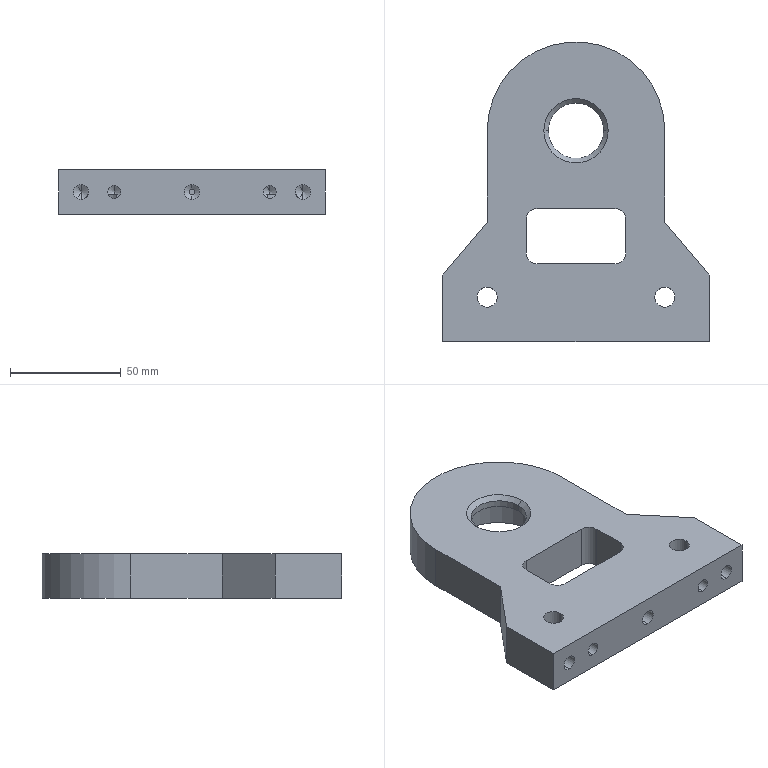Part | SolidWorks | features HoleWzd 3, ICE 2, Chamfer 1, Extrusion 1 | 1 solid | 55 faces | box 120 x 135 x 20 mm | volume 181137 mm3 | cylinder 27 | plane 16 | cone 12 | commonest cylinder face diameters 6.8 x6 6 x4 9 x4 10 x4 15 x4 25 x2